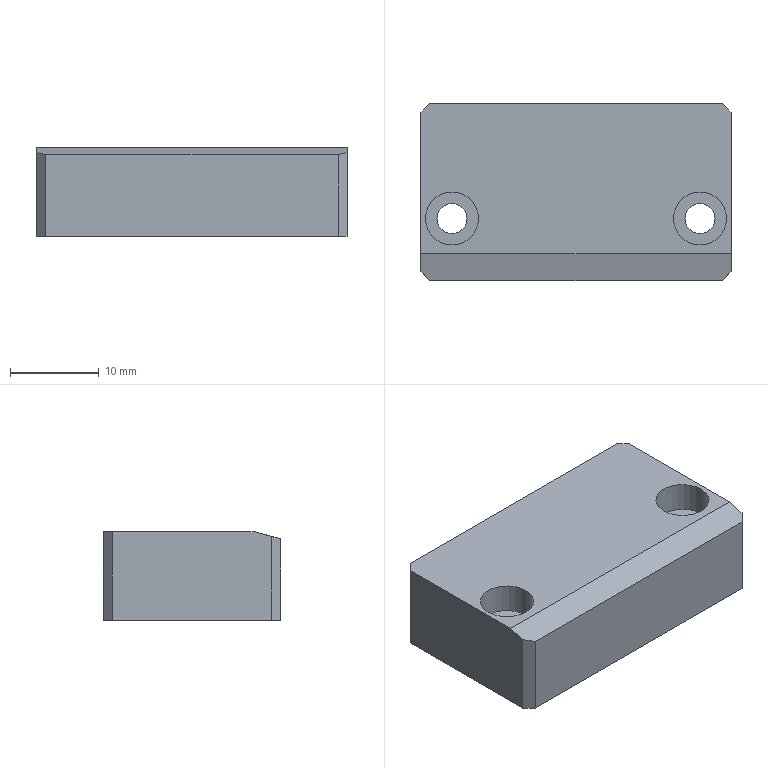Part | STEP file | KF-2212-010-051 | 1 solid | 21 faces | box 35 x 20 x 10 mm | volume 6626 mm3 | plane 13 | cylinder 8 | commonest cylinder face diameters 3.4 x4 6 x4
STEP:
#1=CARTESIAN_POINT('',(11.,-3.,6.6));
#2=VERTEX_POINT('',#1);
#3=CARTESIAN_POINT('',(17.,-3.,6.6));
#4=VERTEX_POINT('',#3);
#5=CARTESIAN_POINT('',(14.,-3.,6.6));
#6=DIRECTION('',(0.,0.,1.));
#7=DIRECTION('',(1.,0.,0.));
#8=AXIS2_PLACEMENT_3D('',#5,#6,#7);
#9=CIRCLE('',#8,3.);
#10=EDGE_CURVE('',#2,#4,#9,.T.);
#11=ORIENTED_EDGE('',*,*,#10,.F.);
#12=CARTESIAN_POINT('',(11.,-3.,10.));
#13=VERTEX_POINT('',#12);
#14=CARTESIAN_POINT('',(11.,-3.,10.));
#15=DIRECTION('',(0.,0.,1.));
#16=VECTOR('',#15,1000.);
#17=LINE('',#14,#16);
#18=EDGE_CURVE('',#2,#13,#17,.T.);
#19=ORIENTED_EDGE('',*,*,#18,.T.);
#20=CARTESIAN_POINT('',(17.,-3.,10.));
#21=VERTEX_POINT('',#20);
#22=CARTESIAN_POINT('',(14.,-3.,10.));
#23=DIRECTION('',(0.,0.,1.));
#24=DIRECTION('',(1.,0.,0.));
#25=AXIS2_PLACEMENT_3D('',#22,#23,#24);
#26=CIRCLE('',#25,3.);
#27=EDGE_CURVE('',#13,#21,#26,.T.);
#28=ORIENTED_EDGE('',*,*,#27,.T.);
#29=CARTESIAN_POINT('',(17.,-3.,10.));
#30=DIRECTION('',(0.,0.,1.));
#31=VECTOR('',#30,1000.);
#32=LINE('',#29,#31);
#33=EDGE_CURVE('',#4,#21,#32,.T.);
#34=ORIENTED_EDGE('',*,*,#33,.F.);
#35=EDGE_LOOP('',(#11,#19,#28,#34));
#36=FACE_OUTER_BOUND('',#35,.T.);
#37=CARTESIAN_POINT('',(14.,-3.,10.));
#38=DIRECTION('',(0.,0.,1.));
#39=DIRECTION('',(1.,0.,0.));
#40=AXIS2_PLACEMENT_3D('',#37,#38,#39);
#41=CYLINDRICAL_SURFACE('',#40,3.);
#42=ADVANCED_FACE('',(#36),#41,.F.);
#43=CARTESIAN_POINT('',(12.3,-3.,0.));
#44=VERTEX_POINT('',#43);
#45=CARTESIAN_POINT('',(15.7,-3.,0.));
#46=VERTEX_POINT('',#45);
#47=CARTESIAN_POINT('',(14.,-3.,0.));
#48=DIRECTION('',(0.,0.,1.));
#49=DIRECTION('',(1.,0.,0.));
#50=AXIS2_PLACEMENT_3D('',#47,#48,#49);
#51=CIRCLE('',#50,1.7);
#52=EDGE_CURVE('',#44,#46,#51,.T.);
#53=ORIENTED_EDGE('',*,*,#52,.F.);
#54=CARTESIAN_POINT('',(12.3,-3.,6.6));
#55=VERTEX_POINT('',#54);
#56=CARTESIAN_POINT('',(12.3,-3.,10.));
#57=DIRECTION('',(0.,0.,1.));
#58=VECTOR('',#57,1000.);
#59=LINE('',#56,#58);
#60=EDGE_CURVE('',#44,#55,#59,.T.);
#61=ORIENTED_EDGE('',*,*,#60,.T.);
#62=CARTESIAN_POINT('',(15.7,-3.,6.6));
#63=VERTEX_POINT('',#62);
#64=CARTESIAN_POINT('',(14.,-3.,6.6));
#65=DIRECTION('',(0.,0.,1.));
#66=DIRECTION('',(1.,0.,0.));
#67=AXIS2_PLACEMENT_3D('',#64,#65,#66);
#68=CIRCLE('',#67,1.7);
#69=EDGE_CURVE('',#55,#63,#68,.T.);
#70=ORIENTED_EDGE('',*,*,#69,.T.);
#71=CARTESIAN_POINT('',(15.7,-3.,10.));
#72=DIRECTION('',(0.,0.,1.));
#73=VECTOR('',#72,1000.);
#74=LINE('',#71,#73);
#75=EDGE_CURVE('',#46,#63,#74,.T.);
#76=ORIENTED_EDGE('',*,*,#75,.F.);
#77=EDGE_LOOP('',(#53,#61,#70,#76));
#78=FACE_OUTER_BOUND('',#77,.T.);
#79=CARTESIAN_POINT('',(14.,-3.,10.));
#80=DIRECTION('',(0.,0.,1.));
#81=DIRECTION('',(1.,0.,0.));
#82=AXIS2_PLACEMENT_3D('',#79,#80,#81);
#83=CYLINDRICAL_SURFACE('',#82,1.7);
#84=ADVANCED_FACE('',(#78),#83,.F.);
#85=CARTESIAN_POINT('',(-17.,-3.,6.6));
#86=VERTEX_POINT('',#85);
#87=CARTESIAN_POINT('',(-11.,-3.,6.6));
#88=VERTEX_POINT('',#87);
#89=CARTESIAN_POINT('',(-14.,-3.,6.6));
#90=DIRECTION('',(0.,0.,1.));
#91=DIRECTION('',(1.,0.,0.));
#92=AXIS2_PLACEMENT_3D('',#89,#90,#91);
#93=CIRCLE('',#92,3.);
#94=EDGE_CURVE('',#86,#88,#93,.T.);
#95=ORIENTED_EDGE('',*,*,#94,.F.);
#96=CARTESIAN_POINT('',(-17.,-3.,10.));
#97=VERTEX_POINT('',#96);
#98=CARTESIAN_POINT('',(-17.,-3.,10.));
#99=DIRECTION('',(0.,0.,1.));
#100=VECTOR('',#99,1000.);
#101=LINE('',#98,#100);
#102=EDGE_CURVE('',#86,#97,#101,.T.);
#103=ORIENTED_EDGE('',*,*,#102,.T.);
#104=CARTESIAN_POINT('',(-11.,-3.,10.));
#105=VERTEX_POINT('',#104);
#106=CARTESIAN_POINT('',(-14.,-3.,10.));
#107=DIRECTION('',(0.,0.,1.));
#108=DIRECTION('',(1.,0.,0.));
#109=AXIS2_PLACEMENT_3D('',#106,#107,#108);
#110=CIRCLE('',#109,3.);
#111=EDGE_CURVE('',#97,#105,#110,.T.);
#112=ORIENTED_EDGE('',*,*,#111,.T.);
#113=CARTESIAN_POINT('',(-11.,-3.,10.));
#114=DIRECTION('',(0.,0.,1.));
#115=VECTOR('',#114,1000.);
#116=LINE('',#113,#115);
#117=EDGE_CURVE('',#88,#105,#116,.T.);
#118=ORIENTED_EDGE('',*,*,#117,.F.);
#119=EDGE_LOOP('',(#95,#103,#112,#118));
#120=FACE_OUTER_BOUND('',#119,.T.);
#121=CARTESIAN_POINT('',(-14.,-3.,10.));
#122=DIRECTION('',(0.,0.,1.));
#123=DIRECTION('',(1.,0.,0.));
#124=AXIS2_PLACEMENT_3D('',#121,#122,#123);
#125=CYLINDRICAL_SURFACE('',#124,3.);
#126=ADVANCED_FACE('',(#120),#125,.F.);
#127=CARTESIAN_POINT('',(-15.7,-3.,0.));
#128=VERTEX_POINT('',#127);
#129=CARTESIAN_POINT('',(-12.3,-3.,0.));
#130=VERTEX_POINT('',#129);
#131=CARTESIAN_POINT('',(-14.,-3.,0.));
#132=DIRECTION('',(0.,0.,1.));
#133=DIRECTION('',(1.,0.,0.));
#134=AXIS2_PLACEMENT_3D('',#131,#132,#133);
#135=CIRCLE('',#134,1.7);
#136=EDGE_CURVE('',#128,#130,#135,.T.);
#137=ORIENTED_EDGE('',*,*,#136,.F.);
#138=CARTESIAN_POINT('',(-15.7,-3.,6.6));
#139=VERTEX_POINT('',#138);
#140=CARTESIAN_POINT('',(-15.7,-3.,10.));
#141=DIRECTION('',(0.,0.,1.));
#142=VECTOR('',#141,1000.);
#143=LINE('',#140,#142);
#144=EDGE_CURVE('',#128,#139,#143,.T.);
#145=ORIENTED_EDGE('',*,*,#144,.T.);
#146=CARTESIAN_POINT('',(-12.3,-3.,6.6));
#147=VERTEX_POINT('',#146);
#148=CARTESIAN_POINT('',(-14.,-3.,6.6));
#149=DIRECTION('',(0.,0.,1.));
#150=DIRECTION('',(1.,0.,0.));
#151=AXIS2_PLACEMENT_3D('',#148,#149,#150);
#152=CIRCLE('',#151,1.7);
#153=EDGE_CURVE('',#139,#147,#152,.T.);
#154=ORIENTED_EDGE('',*,*,#153,.T.);
#155=CARTESIAN_POINT('',(-12.3,-3.,10.));
#156=DIRECTION('',(0.,0.,1.));
#157=VECTOR('',#156,1000.);
#158=LINE('',#155,#157);
#159=EDGE_CURVE('',#130,#147,#158,.T.);
#160=ORIENTED_EDGE('',*,*,#159,.F.);
#161=EDGE_LOOP('',(#137,#145,#154,#160));
#162=FACE_OUTER_BOUND('',#161,.T.);
#163=CARTESIAN_POINT('',(-14.,-3.,10.));
#164=DIRECTION('',(0.,0.,1.));
#165=DIRECTION('',(1.,0.,0.));
#166=AXIS2_PLACEMENT_3D('',#163,#164,#165);
#167=CYLINDRICAL_SURFACE('',#166,1.7);
#168=ADVANCED_FACE('',(#162),#167,.F.);
#169=CARTESIAN_POINT('',(17.5,-7.,10.));
#170=VERTEX_POINT('',#169);
#171=CARTESIAN_POINT('',(17.5,-9.,9.464));
#172=VERTEX_POINT('',#171);
#173=CARTESIAN_POINT('',(17.5,-7.,10.));
#174=DIRECTION('',(0.,-0.9659,-0.2588));
#175=VECTOR('',#174,1000.);
#176=LINE('',#173,#175);
#177=EDGE_CURVE('',#170,#172,#176,.T.);
#178=ORIENTED_EDGE('',*,*,#177,.T.);
#179=CARTESIAN_POINT('',(17.5,-9.,0.));
#180=VERTEX_POINT('',#179);
#181=CARTESIAN_POINT('',(17.5,-9.,10.));
#182=DIRECTION('',(0.,0.,-1.));
#183=VECTOR('',#182,1000.);
#184=LINE('',#181,#183);
#185=EDGE_CURVE('',#172,#180,#184,.T.);
#186=ORIENTED_EDGE('',*,*,#185,.T.);
#187=CARTESIAN_POINT('',(17.5,9.,0.));
#188=VERTEX_POINT('',#187);
#189=CARTESIAN_POINT('',(17.5,10.,0.));
#190=DIRECTION('',(0.,1.,0.));
#191=VECTOR('',#190,1000.);
#192=LINE('',#189,#191);
#193=EDGE_CURVE('',#180,#188,#192,.T.);
#194=ORIENTED_EDGE('',*,*,#193,.T.);
#195=CARTESIAN_POINT('',(17.5,9.,10.));
#196=VERTEX_POINT('',#195);
#197=CARTESIAN_POINT('',(17.5,9.,10.));
#198=DIRECTION('',(0.,0.,1.));
#199=VECTOR('',#198,1000.);
#200=LINE('',#197,#199);
#201=EDGE_CURVE('',#188,#196,#200,.T.);
#202=ORIENTED_EDGE('',*,*,#201,.T.);
#203=CARTESIAN_POINT('',(17.5,10.,10.));
#204=DIRECTION('',(0.,1.,0.));
#205=VECTOR('',#204,1000.);
#206=LINE('',#203,#205);
#207=EDGE_CURVE('',#170,#196,#206,.T.);
#208=ORIENTED_EDGE('',*,*,#207,.F.);
#209=EDGE_LOOP('',(#178,#186,#194,#202,#208));
#210=FACE_OUTER_BOUND('',#209,.T.);
#211=CARTESIAN_POINT('',(17.5,10.,10.));
#212=DIRECTION('',(-1.,0.,0.));
#213=DIRECTION('',(0.,0.,1.));
#214=AXIS2_PLACEMENT_3D('',#211,#212,#213);
#215=PLANE('',#214);
#216=ADVANCED_FACE('',(#210),#215,.F.);
#217=CARTESIAN_POINT('',(16.5,10.,10.));
#218=VERTEX_POINT('',#217);
#219=CARTESIAN_POINT('',(-16.5,10.,10.));
#220=VERTEX_POINT('',#219);
#221=CARTESIAN_POINT('',(-17.5,10.,10.));
#222=DIRECTION('',(-1.,0.,0.));
#223=VECTOR('',#222,1000.);
#224=LINE('',#221,#223);
#225=EDGE_CURVE('',#218,#220,#224,.T.);
#226=ORIENTED_EDGE('',*,*,#225,.F.);
#227=CARTESIAN_POINT('',(16.5,10.,0.));
#228=VERTEX_POINT('',#227);
#229=CARTESIAN_POINT('',(16.5,10.,10.));
#230=DIRECTION('',(0.,0.,-1.));
#231=VECTOR('',#230,1000.);
#232=LINE('',#229,#231);
#233=EDGE_CURVE('',#218,#228,#232,.T.);
#234=ORIENTED_EDGE('',*,*,#233,.T.);
#235=CARTESIAN_POINT('',(-16.5,10.,0.));
#236=VERTEX_POINT('',#235);
#237=CARTESIAN_POINT('',(-17.5,10.,0.));
#238=DIRECTION('',(-1.,0.,0.));
#239=VECTOR('',#238,1000.);
#240=LINE('',#237,#239);
#241=EDGE_CURVE('',#228,#236,#240,.T.);
#242=ORIENTED_EDGE('',*,*,#241,.T.);
#243=CARTESIAN_POINT('',(-16.5,10.,10.));
#244=DIRECTION('',(0.,0.,1.));
#245=VECTOR('',#244,1000.);
#246=LINE('',#243,#245);
#247=EDGE_CURVE('',#236,#220,#246,.T.);
#248=ORIENTED_EDGE('',*,*,#247,.T.);
#249=EDGE_LOOP('',(#226,#234,#242,#248));
#250=FACE_OUTER_BOUND('',#249,.T.);
#251=CARTESIAN_POINT('',(-17.5,10.,10.));
#252=DIRECTION('',(0.,-1.,0.));
#253=DIRECTION('',(1.,0.,0.));
#254=AXIS2_PLACEMENT_3D('',#251,#252,#253);
#255=PLANE('',#254);
#256=ADVANCED_FACE('',(#250),#255,.F.);
#257=CARTESIAN_POINT('',(-17.5,9.,0.));
#258=VERTEX_POINT('',#257);
#259=CARTESIAN_POINT('',(-17.5,-9.,0.));
#260=VERTEX_POINT('',#259);
#261=CARTESIAN_POINT('',(-17.5,10.,0.));
#262=DIRECTION('',(0.,-1.,0.));
#263=VECTOR('',#262,1000.);
#264=LINE('',#261,#263);
#265=EDGE_CURVE('',#258,#260,#264,.T.);
#266=ORIENTED_EDGE('',*,*,#265,.T.);
#267=CARTESIAN_POINT('',(-17.5,-9.,9.464));
#268=VERTEX_POINT('',#267);
#269=CARTESIAN_POINT('',(-17.5,-9.,10.));
#270=DIRECTION('',(0.,0.,1.));
#271=VECTOR('',#270,1000.);
#272=LINE('',#269,#271);
#273=EDGE_CURVE('',#260,#268,#272,.T.);
#274=ORIENTED_EDGE('',*,*,#273,.T.);
#275=CARTESIAN_POINT('',(-17.5,-7.,10.));
#276=VERTEX_POINT('',#275);
#277=CARTESIAN_POINT('',(-17.5,-7.,10.));
#278=DIRECTION('',(0.,0.9659,0.2588));
#279=VECTOR('',#278,1000.);
#280=LINE('',#277,#279);
#281=EDGE_CURVE('',#268,#276,#280,.T.);
#282=ORIENTED_EDGE('',*,*,#281,.T.);
#283=CARTESIAN_POINT('',(-17.5,9.,10.));
#284=VERTEX_POINT('',#283);
#285=CARTESIAN_POINT('',(-17.5,10.,10.));
#286=DIRECTION('',(0.,-1.,0.));
#287=VECTOR('',#286,1000.);
#288=LINE('',#285,#287);
#289=EDGE_CURVE('',#284,#276,#288,.T.);
#290=ORIENTED_EDGE('',*,*,#289,.F.);
#291=CARTESIAN_POINT('',(-17.5,9.,10.));
#292=DIRECTION('',(0.,0.,-1.));
#293=VECTOR('',#292,1000.);
#294=LINE('',#291,#293);
#295=EDGE_CURVE('',#284,#258,#294,.T.);
#296=ORIENTED_EDGE('',*,*,#295,.T.);
#297=EDGE_LOOP('',(#266,#274,#282,#290,#296));
#298=FACE_OUTER_BOUND('',#297,.T.);
#299=CARTESIAN_POINT('',(-17.5,10.,10.));
#300=DIRECTION('',(1.,0.,0.));
#301=DIRECTION('',(0.,1.,0.));
#302=AXIS2_PLACEMENT_3D('',#299,#300,#301);
#303=PLANE('',#302);
#304=ADVANCED_FACE('',(#298),#303,.F.);
#305=CARTESIAN_POINT('',(-16.5,-10.,0.));
#306=VERTEX_POINT('',#305);
#307=CARTESIAN_POINT('',(16.5,-10.,0.));
#308=VERTEX_POINT('',#307);
#309=CARTESIAN_POINT('',(-17.5,-10.,0.));
#310=DIRECTION('',(1.,0.,0.));
#311=VECTOR('',#310,1000.);
#312=LINE('',#309,#311);
#313=EDGE_CURVE('',#306,#308,#312,.T.);
#314=ORIENTED_EDGE('',*,*,#313,.T.);
#315=CARTESIAN_POINT('',(16.5,-10.,9.196));
#316=VERTEX_POINT('',#315);
#317=CARTESIAN_POINT('',(16.5,-10.,10.));
#318=DIRECTION('',(0.,0.,1.));
#319=VECTOR('',#318,1000.);
#320=LINE('',#317,#319);
#321=EDGE_CURVE('',#308,#316,#320,.T.);
#322=ORIENTED_EDGE('',*,*,#321,.T.);
#323=CARTESIAN_POINT('',(-16.5,-10.,9.196));
#324=VERTEX_POINT('',#323);
#325=CARTESIAN_POINT('',(-17.5,-10.,9.196));
#326=DIRECTION('',(-1.,0.,0.));
#327=VECTOR('',#326,1000.);
#328=LINE('',#325,#327);
#329=EDGE_CURVE('',#316,#324,#328,.T.);
#330=ORIENTED_EDGE('',*,*,#329,.T.);
#331=CARTESIAN_POINT('',(-16.5,-10.,10.));
#332=DIRECTION('',(0.,0.,-1.));
#333=VECTOR('',#332,1000.);
#334=LINE('',#331,#333);
#335=EDGE_CURVE('',#324,#306,#334,.T.);
#336=ORIENTED_EDGE('',*,*,#335,.T.);
#337=EDGE_LOOP('',(#314,#322,#330,#336));
#338=FACE_OUTER_BOUND('',#337,.T.);
#339=CARTESIAN_POINT('',(-17.5,-10.,10.));
#340=DIRECTION('',(0.,1.,0.));
#341=DIRECTION('',(-1.,0.,0.));
#342=AXIS2_PLACEMENT_3D('',#339,#340,#341);
#343=PLANE('',#342);
#344=ADVANCED_FACE('',(#338),#343,.F.);
#345=CARTESIAN_POINT('',(14.,-3.,10.));
#346=DIRECTION('',(0.,0.,1.));
#347=DIRECTION('',(1.,0.,0.));
#348=AXIS2_PLACEMENT_3D('',#345,#346,#347);
#349=CIRCLE('',#348,3.);
#350=EDGE_CURVE('',#21,#13,#349,.T.);
#351=ORIENTED_EDGE('',*,*,#350,.F.);
#352=ORIENTED_EDGE('',*,*,#27,.F.);
#353=EDGE_LOOP('',(#351,#352));
#354=FACE_BOUND('',#353,.T.);
#355=CARTESIAN_POINT('',(-14.,-3.,10.));
#356=DIRECTION('',(0.,0.,1.));
#357=DIRECTION('',(1.,0.,0.));
#358=AXIS2_PLACEMENT_3D('',#355,#356,#357);
#359=CIRCLE('',#358,3.);
#360=EDGE_CURVE('',#105,#97,#359,.T.);
#361=ORIENTED_EDGE('',*,*,#360,.F.);
#362=ORIENTED_EDGE('',*,*,#111,.F.);
#363=EDGE_LOOP('',(#361,#362));
#364=FACE_BOUND('',#363,.T.);
#365=ORIENTED_EDGE('',*,*,#207,.T.);
#366=CARTESIAN_POINT('',(13.25,13.25,10.));
#367=DIRECTION('',(-0.7071,0.7071,0.));
#368=VECTOR('',#367,1000.);
#369=LINE('',#366,#368);
#370=EDGE_CURVE('',#196,#218,#369,.T.);
#371=ORIENTED_EDGE('',*,*,#370,.T.);
#372=ORIENTED_EDGE('',*,*,#225,.T.);
#373=CARTESIAN_POINT('',(-13.25,13.25,10.));
#374=DIRECTION('',(-0.7071,-0.7071,0.));
#375=VECTOR('',#374,1000.);
#376=LINE('',#373,#375);
#377=EDGE_CURVE('',#220,#284,#376,.T.);
#378=ORIENTED_EDGE('',*,*,#377,.T.);
#379=ORIENTED_EDGE('',*,*,#289,.T.);
#380=CARTESIAN_POINT('',(17.5,-7.,10.));
#381=DIRECTION('',(1.,0.,0.));
#382=VECTOR('',#381,1000.);
#383=LINE('',#380,#382);
#384=EDGE_CURVE('',#276,#170,#383,.T.);
#385=ORIENTED_EDGE('',*,*,#384,.T.);
#386=EDGE_LOOP('',(#365,#371,#372,#378,#379,#385));
#387=FACE_OUTER_BOUND('',#386,.T.);
#388=CARTESIAN_POINT('',(0.,0.,10.));
#389=DIRECTION('',(0.,0.,1.));
#390=DIRECTION('',(1.,0.,0.));
#391=AXIS2_PLACEMENT_3D('',#388,#389,#390);
#392=PLANE('',#391);
#393=ADVANCED_FACE('',(#354,#364,#387),#392,.T.);
#394=CARTESIAN_POINT('',(14.,-3.,0.));
#395=DIRECTION('',(0.,0.,1.));
#396=DIRECTION('',(1.,0.,0.));
#397=AXIS2_PLACEMENT_3D('',#394,#395,#396);
#398=CIRCLE('',#397,1.7);
#399=EDGE_CURVE('',#46,#44,#398,.T.);
#400=ORIENTED_EDGE('',*,*,#399,.T.);
#401=ORIENTED_EDGE('',*,*,#52,.T.);
#402=EDGE_LOOP('',(#400,#401));
#403=FACE_BOUND('',#402,.T.);
#404=CARTESIAN_POINT('',(-14.,-3.,0.));
#405=DIRECTION('',(0.,0.,1.));
#406=DIRECTION('',(1.,0.,0.));
#407=AXIS2_PLACEMENT_3D('',#404,#405,#406);
#408=CIRCLE('',#407,1.7);
#409=EDGE_CURVE('',#130,#128,#408,.T.);
#410=ORIENTED_EDGE('',*,*,#409,.T.);
#411=ORIENTED_EDGE('',*,*,#136,.T.);
#412=EDGE_LOOP('',(#410,#411));
#413=FACE_BOUND('',#412,.T.);
#414=ORIENTED_EDGE('',*,*,#193,.F.);
#415=CARTESIAN_POINT('',(17.5,-9.,0.));
#416=DIRECTION('',(-0.7071,-0.7071,0.));
#417=VECTOR('',#416,1000.);
#418=LINE('',#415,#417);
#419=EDGE_CURVE('',#180,#308,#418,.T.);
#420=ORIENTED_EDGE('',*,*,#419,.T.);
#421=ORIENTED_EDGE('',*,*,#313,.F.);
#422=CARTESIAN_POINT('',(-16.5,-10.,0.));
#423=DIRECTION('',(-0.7071,0.7071,0.));
#424=VECTOR('',#423,1000.);
#425=LINE('',#422,#424);
#426=EDGE_CURVE('',#306,#260,#425,.T.);
#427=ORIENTED_EDGE('',*,*,#426,.T.);
#428=ORIENTED_EDGE('',*,*,#265,.F.);
#429=CARTESIAN_POINT('',(-17.5,9.,0.));
#430=DIRECTION('',(0.7071,0.7071,0.));
#431=VECTOR('',#430,1000.);
#432=LINE('',#429,#431);
#433=EDGE_CURVE('',#258,#236,#432,.T.);
#434=ORIENTED_EDGE('',*,*,#433,.T.);
#435=ORIENTED_EDGE('',*,*,#241,.F.);
#436=CARTESIAN_POINT('',(16.5,10.,0.));
#437=DIRECTION('',(0.7071,-0.7071,0.));
#438=VECTOR('',#437,1000.);
#439=LINE('',#436,#438);
#440=EDGE_CURVE('',#228,#188,#439,.T.);
#441=ORIENTED_EDGE('',*,*,#440,.T.);
#442=EDGE_LOOP('',(#414,#420,#421,#427,#428,#434,#435,#441));
#443=FACE_OUTER_BOUND('',#442,.T.);
#444=CARTESIAN_POINT('',(0.,0.,0.));
#445=DIRECTION('',(0.,0.,1.));
#446=DIRECTION('',(1.,0.,0.));
#447=AXIS2_PLACEMENT_3D('',#444,#445,#446);
#448=PLANE('',#447);
#449=ADVANCED_FACE('',(#403,#413,#443),#448,.F.);
#450=ORIENTED_EDGE('',*,*,#144,.F.);
#451=ORIENTED_EDGE('',*,*,#409,.F.);
#452=ORIENTED_EDGE('',*,*,#159,.T.);
#453=CARTESIAN_POINT('',(-14.,-3.,6.6));
#454=DIRECTION('',(0.,0.,1.));
#455=DIRECTION('',(1.,0.,0.));
#456=AXIS2_PLACEMENT_3D('',#453,#454,#455);
#457=CIRCLE('',#456,1.7);
#458=EDGE_CURVE('',#147,#139,#457,.T.);
#459=ORIENTED_EDGE('',*,*,#458,.T.);
#460=EDGE_LOOP('',(#450,#451,#452,#459));
#461=FACE_OUTER_BOUND('',#460,.T.);
#462=CARTESIAN_POINT('',(-14.,-3.,10.));
#463=DIRECTION('',(0.,0.,1.));
#464=DIRECTION('',(1.,0.,0.));
#465=AXIS2_PLACEMENT_3D('',#462,#463,#464);
#466=CYLINDRICAL_SURFACE('',#465,1.7);
#467=ADVANCED_FACE('',(#461),#466,.F.);
#468=ORIENTED_EDGE('',*,*,#458,.F.);
#469=ORIENTED_EDGE('',*,*,#153,.F.);
#470=EDGE_LOOP('',(#468,#469));
#471=FACE_BOUND('',#470,.T.);
#472=CARTESIAN_POINT('',(-14.,-3.,6.6));
#473=DIRECTION('',(0.,0.,1.));
#474=DIRECTION('',(1.,0.,0.));
#475=AXIS2_PLACEMENT_3D('',#472,#473,#474);
#476=CIRCLE('',#475,3.);
#477=EDGE_CURVE('',#88,#86,#476,.T.);
#478=ORIENTED_EDGE('',*,*,#477,.T.);
#479=ORIENTED_EDGE('',*,*,#94,.T.);
#480=EDGE_LOOP('',(#478,#479));
#481=FACE_OUTER_BOUND('',#480,.T.);
#482=CARTESIAN_POINT('',(-12.3,-3.,6.6));
#483=DIRECTION('',(0.,0.,-1.));
#484=DIRECTION('',(-1.,0.,0.));
#485=AXIS2_PLACEMENT_3D('',#482,#483,#484);
#486=PLANE('',#485);
#487=ADVANCED_FACE('',(#471,#481),#486,.F.);
#488=ORIENTED_EDGE('',*,*,#102,.F.);
#489=ORIENTED_EDGE('',*,*,#477,.F.);
#490=ORIENTED_EDGE('',*,*,#117,.T.);
#491=ORIENTED_EDGE('',*,*,#360,.T.);
#492=EDGE_LOOP('',(#488,#489,#490,#491));
#493=FACE_OUTER_BOUND('',#492,.T.);
#494=CARTESIAN_POINT('',(-14.,-3.,10.));
#495=DIRECTION('',(0.,0.,1.));
#496=DIRECTION('',(1.,0.,0.));
#497=AXIS2_PLACEMENT_3D('',#494,#495,#496);
#498=CYLINDRICAL_SURFACE('',#497,3.);
#499=ADVANCED_FACE('',(#493),#498,.F.);
#500=ORIENTED_EDGE('',*,*,#60,.F.);
#501=ORIENTED_EDGE('',*,*,#399,.F.);
#502=ORIENTED_EDGE('',*,*,#75,.T.);
#503=CARTESIAN_POINT('',(14.,-3.,6.6));
#504=DIRECTION('',(0.,0.,1.));
#505=DIRECTION('',(1.,0.,0.));
#506=AXIS2_PLACEMENT_3D('',#503,#504,#505);
#507=CIRCLE('',#506,1.7);
#508=EDGE_CURVE('',#63,#55,#507,.T.);
#509=ORIENTED_EDGE('',*,*,#508,.T.);
#510=EDGE_LOOP('',(#500,#501,#502,#509));
#511=FACE_OUTER_BOUND('',#510,.T.);
#512=CARTESIAN_POINT('',(14.,-3.,10.));
#513=DIRECTION('',(0.,0.,1.));
#514=DIRECTION('',(1.,0.,0.));
#515=AXIS2_PLACEMENT_3D('',#512,#513,#514);
#516=CYLINDRICAL_SURFACE('',#515,1.7);
#517=ADVANCED_FACE('',(#511),#516,.F.);
#518=ORIENTED_EDGE('',*,*,#508,.F.);
#519=ORIENTED_EDGE('',*,*,#69,.F.);
#520=EDGE_LOOP('',(#518,#519));
#521=FACE_BOUND('',#520,.T.);
#522=CARTESIAN_POINT('',(14.,-3.,6.6));
#523=DIRECTION('',(0.,0.,1.));
#524=DIRECTION('',(1.,0.,0.));
#525=AXIS2_PLACEMENT_3D('',#522,#523,#524);
#526=CIRCLE('',#525,3.);
#527=EDGE_CURVE('',#4,#2,#526,.T.);
#528=ORIENTED_EDGE('',*,*,#527,.T.);
#529=ORIENTED_EDGE('',*,*,#10,.T.);
#530=EDGE_LOOP('',(#528,#529));
#531=FACE_OUTER_BOUND('',#530,.T.);
#532=CARTESIAN_POINT('',(15.7,-3.,6.6));
#533=DIRECTION('',(0.,0.,-1.));
#534=DIRECTION('',(-1.,0.,0.));
#535=AXIS2_PLACEMENT_3D('',#532,#533,#534);
#536=PLANE('',#535);
#537=ADVANCED_FACE('',(#521,#531),#536,.F.);
#538=ORIENTED_EDGE('',*,*,#18,.F.);
#539=ORIENTED_EDGE('',*,*,#527,.F.);
#540=ORIENTED_EDGE('',*,*,#33,.T.);
#541=ORIENTED_EDGE('',*,*,#350,.T.);
#542=EDGE_LOOP('',(#538,#539,#540,#541));
#543=FACE_OUTER_BOUND('',#542,.T.);
#544=CARTESIAN_POINT('',(14.,-3.,10.));
#545=DIRECTION('',(0.,0.,1.));
#546=DIRECTION('',(1.,0.,0.));
#547=AXIS2_PLACEMENT_3D('',#544,#545,#546);
#548=CYLINDRICAL_SURFACE('',#547,3.);
#549=ADVANCED_FACE('',(#543),#548,.F.);
#550=ORIENTED_EDGE('',*,*,#329,.F.);
#551=CARTESIAN_POINT('',(10.088,-16.412,7.478));
#552=DIRECTION('',(0.6947,0.6947,0.1862));
#553=VECTOR('',#552,1000.);
#554=LINE('',#551,#553);
#555=EDGE_CURVE('',#316,#172,#554,.T.);
#556=ORIENTED_EDGE('',*,*,#555,.T.);
#557=ORIENTED_EDGE('',*,*,#177,.F.);
#558=ORIENTED_EDGE('',*,*,#384,.F.);
#559=ORIENTED_EDGE('',*,*,#281,.F.);
#560=CARTESIAN_POINT('',(-10.088,-16.412,7.478));
#561=DIRECTION('',(0.6947,-0.6947,-0.1862));
#562=VECTOR('',#561,1000.);
#563=LINE('',#560,#562);
#564=EDGE_CURVE('',#268,#324,#563,.T.);
#565=ORIENTED_EDGE('',*,*,#564,.T.);
#566=EDGE_LOOP('',(#550,#556,#557,#558,#559,#565));
#567=FACE_OUTER_BOUND('',#566,.T.);
#568=CARTESIAN_POINT('',(0.,-7.,10.));
#569=DIRECTION('',(0.,-0.2588,0.9659));
#570=DIRECTION('',(-1.,0.,0.));
#571=AXIS2_PLACEMENT_3D('',#568,#569,#570);
#572=PLANE('',#571);
#573=ADVANCED_FACE('',(#567),#572,.T.);
#574=ORIENTED_EDGE('',*,*,#555,.F.);
#575=ORIENTED_EDGE('',*,*,#321,.F.);
#576=ORIENTED_EDGE('',*,*,#419,.F.);
#577=ORIENTED_EDGE('',*,*,#185,.F.);
#578=EDGE_LOOP('',(#574,#575,#576,#577));
#579=FACE_OUTER_BOUND('',#578,.T.);
#580=CARTESIAN_POINT('',(17.5,-9.,10.));
#581=DIRECTION('',(-0.7071,0.7071,0.));
#582=DIRECTION('',(0.,0.,-1.));
#583=AXIS2_PLACEMENT_3D('',#580,#581,#582);
#584=PLANE('',#583);
#585=ADVANCED_FACE('',(#579),#584,.F.);
#586=ORIENTED_EDGE('',*,*,#564,.F.);
#587=ORIENTED_EDGE('',*,*,#273,.F.);
#588=ORIENTED_EDGE('',*,*,#426,.F.);
#589=ORIENTED_EDGE('',*,*,#335,.F.);
#590=EDGE_LOOP('',(#586,#587,#588,#589));
#591=FACE_OUTER_BOUND('',#590,.T.);
#592=CARTESIAN_POINT('',(-16.5,-10.,10.));
#593=DIRECTION('',(0.7071,0.7071,0.));
#594=DIRECTION('',(0.,0.,-1.));
#595=AXIS2_PLACEMENT_3D('',#592,#593,#594);
#596=PLANE('',#595);
#597=ADVANCED_FACE('',(#591),#596,.F.);
#598=ORIENTED_EDGE('',*,*,#370,.F.);
#599=ORIENTED_EDGE('',*,*,#201,.F.);
#600=ORIENTED_EDGE('',*,*,#440,.F.);
#601=ORIENTED_EDGE('',*,*,#233,.F.);
#602=EDGE_LOOP('',(#598,#599,#600,#601));
#603=FACE_OUTER_BOUND('',#602,.T.);
#604=CARTESIAN_POINT('',(16.5,10.,10.));
#605=DIRECTION('',(-0.7071,-0.7071,0.));
#606=DIRECTION('',(0.,0.,-1.));
#607=AXIS2_PLACEMENT_3D('',#604,#605,#606);
#608=PLANE('',#607);
#609=ADVANCED_FACE('',(#603),#608,.F.);
#610=ORIENTED_EDGE('',*,*,#377,.F.);
#611=ORIENTED_EDGE('',*,*,#247,.F.);
#612=ORIENTED_EDGE('',*,*,#433,.F.);
#613=ORIENTED_EDGE('',*,*,#295,.F.);
#614=EDGE_LOOP('',(#610,#611,#612,#613));
#615=FACE_OUTER_BOUND('',#614,.T.);
#616=CARTESIAN_POINT('',(-17.5,9.,10.));
#617=DIRECTION('',(0.7071,-0.7071,0.));
#618=DIRECTION('',(0.,0.,-1.));
#619=AXIS2_PLACEMENT_3D('',#616,#617,#618);
#620=PLANE('',#619);
#621=ADVANCED_FACE('',(#615),#620,.F.);
#622=CLOSED_SHELL('',(#42,#84,#126,#168,#216,#256,#304,#344,#393,#449,#467,#487,#499,#517,#537,#549,#573,#585,#597,#609,#621));
#623=MANIFOLD_SOLID_BREP('',#622);
#624=CARTESIAN_POINT('',(0.,0.,0.));
#625=DIRECTION('',(0.,0.,1.));
#626=DIRECTION('',(1.,0.,0.));
#627=AXIS2_PLACEMENT_3D('',#624,#625,#626);
#628=(LENGTH_UNIT()NAMED_UNIT(*)SI_UNIT(.MILLI.,.METRE.));
#629=UNCERTAINTY_MEASURE_WITH_UNIT(LENGTH_MEASURE(0.00001),#628,'','');
#630=(NAMED_UNIT(*)PLANE_ANGLE_UNIT()SI_UNIT($,.RADIAN.));
#631=(NAMED_UNIT(*)SI_UNIT($,.STERADIAN.)SOLID_ANGLE_UNIT());
#632=(GEOMETRIC_REPRESENTATION_CONTEXT(3)GLOBAL_UNCERTAINTY_ASSIGNED_CONTEXT((#629))GLOBAL_UNIT_ASSIGNED_CONTEXT((#628,#630,#631))REPRESENTATION_CONTEXT('',''));
#633=ADVANCED_BREP_SHAPE_REPRESENTATION('',(#623,#627),#632);